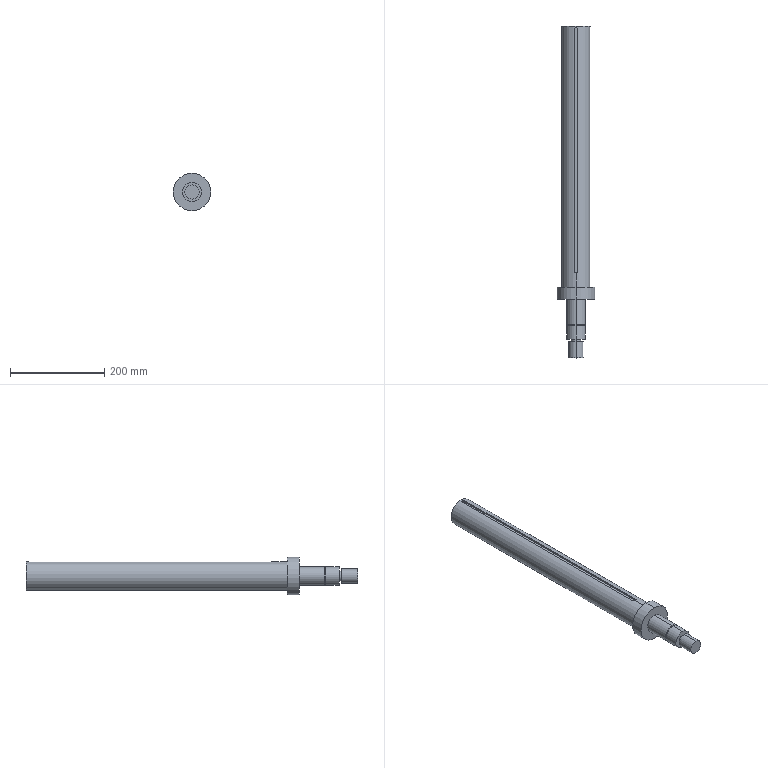Part | SolidWorks | features ICE 3, Revolution 1 | 1 solid | 30 faces | box 80 x 705.59 x 80 mm | volume 1778352 mm3 | cylinder 18 | plane 12 | commonest cylinder face diameters 30 x4 40 x4 8 x2 20 x2 36 x2 60 x2
STEP:
#1=CARTESIAN_POINT('',(0.,411.976,-15.));
#2=VERTEX_POINT('',#1);
#3=CARTESIAN_POINT('',(0.,411.976,15.));
#4=VERTEX_POINT('',#3);
#5=CARTESIAN_POINT('',(0.,411.976,0.));
#6=DIRECTION('',(0.,1.,0.));
#7=DIRECTION('',(0.,0.,1.));
#8=AXIS2_PLACEMENT_3D('',#5,#6,#7);
#9=CIRCLE('',#8,15.);
#10=EDGE_CURVE('',#2,#4,#9,.T.);
#11=ORIENTED_EDGE('',*,*,#10,.F.);
#12=CARTESIAN_POINT('',(0.,461.976,-15.));
#13=VERTEX_POINT('',#12);
#14=CARTESIAN_POINT('',(0.,411.976,-15.));
#15=DIRECTION('',(0.,1.,0.));
#16=VECTOR('',#15,1000.);
#17=LINE('',#14,#16);
#18=EDGE_CURVE('',#2,#13,#17,.T.);
#19=ORIENTED_EDGE('',*,*,#18,.T.);
#20=CARTESIAN_POINT('',(0.,461.976,15.));
#21=VERTEX_POINT('',#20);
#22=CARTESIAN_POINT('',(0.,461.976,0.));
#23=DIRECTION('',(0.,1.,0.));
#24=DIRECTION('',(0.,0.,1.));
#25=AXIS2_PLACEMENT_3D('',#22,#23,#24);
#26=CIRCLE('',#25,15.);
#27=EDGE_CURVE('',#13,#21,#26,.T.);
#28=ORIENTED_EDGE('',*,*,#27,.T.);
#29=CARTESIAN_POINT('',(0.,411.976,15.));
#30=DIRECTION('',(0.,1.,0.));
#31=VECTOR('',#30,1000.);
#32=LINE('',#29,#31);
#33=EDGE_CURVE('',#4,#21,#32,.T.);
#34=ORIENTED_EDGE('',*,*,#33,.F.);
#35=EDGE_LOOP('',(#11,#19,#28,#34));
#36=FACE_OUTER_BOUND('',#35,.T.);
#37=CARTESIAN_POINT('',(0.,411.976,0.));
#38=DIRECTION('',(0.,1.,0.));
#39=DIRECTION('',(0.,0.,1.));
#40=AXIS2_PLACEMENT_3D('',#37,#38,#39);
#41=CYLINDRICAL_SURFACE('',#40,15.);
#42=ADVANCED_FACE('',(#36),#41,.F.);
#43=CARTESIAN_POINT('',(0.,-118.614,40.));
#44=VERTEX_POINT('',#43);
#45=CARTESIAN_POINT('',(0.,-118.614,-40.));
#46=VERTEX_POINT('',#45);
#47=CARTESIAN_POINT('',(0.,-118.614,0.));
#48=DIRECTION('',(0.,1.,0.));
#49=DIRECTION('',(0.,0.,1.));
#50=AXIS2_PLACEMENT_3D('',#47,#48,#49);
#51=CIRCLE('',#50,40.);
#52=EDGE_CURVE('',#44,#46,#51,.T.);
#53=ORIENTED_EDGE('',*,*,#52,.T.);
#54=CARTESIAN_POINT('',(0.,-93.614,-40.));
#55=VERTEX_POINT('',#54);
#56=CARTESIAN_POINT('',(0.,247.86,-40.));
#57=DIRECTION('',(0.,1.,0.));
#58=VECTOR('',#57,1000.);
#59=LINE('',#56,#58);
#60=EDGE_CURVE('',#46,#55,#59,.T.);
#61=ORIENTED_EDGE('',*,*,#60,.T.);
#62=CARTESIAN_POINT('',(0.,-93.614,40.));
#63=VERTEX_POINT('',#62);
#64=CARTESIAN_POINT('',(0.,-93.614,0.));
#65=DIRECTION('',(0.,1.,0.));
#66=DIRECTION('',(0.,0.,1.));
#67=AXIS2_PLACEMENT_3D('',#64,#65,#66);
#68=CIRCLE('',#67,40.);
#69=EDGE_CURVE('',#63,#55,#68,.T.);
#70=ORIENTED_EDGE('',*,*,#69,.F.);
#71=CARTESIAN_POINT('',(0.,247.86,40.));
#72=DIRECTION('',(0.,1.,0.));
#73=VECTOR('',#72,1000.);
#74=LINE('',#71,#73);
#75=EDGE_CURVE('',#44,#63,#74,.T.);
#76=ORIENTED_EDGE('',*,*,#75,.F.);
#77=EDGE_LOOP('',(#53,#61,#70,#76));
#78=FACE_OUTER_BOUND('',#77,.T.);
#79=CARTESIAN_POINT('',(0.,247.86,0.));
#80=DIRECTION('',(0.,1.,0.));
#81=DIRECTION('',(0.,0.,1.));
#82=AXIS2_PLACEMENT_3D('',#79,#80,#81);
#83=CYLINDRICAL_SURFACE('',#82,40.);
#84=ADVANCED_FACE('',(#78),#83,.T.);
#85=CARTESIAN_POINT('',(0.,-171.914,20.));
#86=VERTEX_POINT('',#85);
#87=CARTESIAN_POINT('',(0.,-171.914,-20.));
#88=VERTEX_POINT('',#87);
#89=CARTESIAN_POINT('',(0.,-171.914,0.));
#90=DIRECTION('',(0.,1.,0.));
#91=DIRECTION('',(0.,0.,1.));
#92=AXIS2_PLACEMENT_3D('',#89,#90,#91);
#93=CIRCLE('',#92,20.);
#94=EDGE_CURVE('',#86,#88,#93,.T.);
#95=ORIENTED_EDGE('',*,*,#94,.T.);
#96=CARTESIAN_POINT('',(0.,-118.614,-20.));
#97=VERTEX_POINT('',#96);
#98=CARTESIAN_POINT('',(0.,247.86,-20.));
#99=DIRECTION('',(0.,1.,0.));
#100=VECTOR('',#99,1000.);
#101=LINE('',#98,#100);
#102=EDGE_CURVE('',#88,#97,#101,.T.);
#103=ORIENTED_EDGE('',*,*,#102,.T.);
#104=CARTESIAN_POINT('',(0.,-118.614,20.));
#105=VERTEX_POINT('',#104);
#106=CARTESIAN_POINT('',(0.,-118.614,0.));
#107=DIRECTION('',(0.,1.,0.));
#108=DIRECTION('',(0.,0.,1.));
#109=AXIS2_PLACEMENT_3D('',#106,#107,#108);
#110=CIRCLE('',#109,20.);
#111=EDGE_CURVE('',#105,#97,#110,.T.);
#112=ORIENTED_EDGE('',*,*,#111,.F.);
#113=CARTESIAN_POINT('',(0.,247.86,20.));
#114=DIRECTION('',(0.,1.,0.));
#115=VECTOR('',#114,1000.);
#116=LINE('',#113,#115);
#117=EDGE_CURVE('',#86,#105,#116,.T.);
#118=ORIENTED_EDGE('',*,*,#117,.F.);
#119=EDGE_LOOP('',(#95,#103,#112,#118));
#120=FACE_OUTER_BOUND('',#119,.T.);
#121=CARTESIAN_POINT('',(0.,247.86,0.));
#122=DIRECTION('',(0.,1.,0.));
#123=DIRECTION('',(0.,0.,1.));
#124=AXIS2_PLACEMENT_3D('',#121,#122,#123);
#125=CYLINDRICAL_SURFACE('',#124,20.);
#126=ADVANCED_FACE('',(#120),#125,.T.);
#127=CARTESIAN_POINT('',(0.,-174.914,18.));
#128=VERTEX_POINT('',#127);
#129=CARTESIAN_POINT('',(0.,-174.914,-18.));
#130=VERTEX_POINT('',#129);
#131=CARTESIAN_POINT('',(0.,-174.914,0.));
#132=DIRECTION('',(0.,1.,0.));
#133=DIRECTION('',(0.,0.,1.));
#134=AXIS2_PLACEMENT_3D('',#131,#132,#133);
#135=CIRCLE('',#134,18.);
#136=EDGE_CURVE('',#128,#130,#135,.T.);
#137=ORIENTED_EDGE('',*,*,#136,.T.);
#138=CARTESIAN_POINT('',(0.,-171.914,-18.));
#139=VERTEX_POINT('',#138);
#140=CARTESIAN_POINT('',(0.,247.86,-18.));
#141=DIRECTION('',(0.,1.,0.));
#142=VECTOR('',#141,1000.);
#143=LINE('',#140,#142);
#144=EDGE_CURVE('',#130,#139,#143,.T.);
#145=ORIENTED_EDGE('',*,*,#144,.T.);
#146=CARTESIAN_POINT('',(0.,-171.914,18.));
#147=VERTEX_POINT('',#146);
#148=CARTESIAN_POINT('',(0.,-171.914,0.));
#149=DIRECTION('',(0.,1.,0.));
#150=DIRECTION('',(0.,0.,1.));
#151=AXIS2_PLACEMENT_3D('',#148,#149,#150);
#152=CIRCLE('',#151,18.);
#153=EDGE_CURVE('',#147,#139,#152,.T.);
#154=ORIENTED_EDGE('',*,*,#153,.F.);
#155=CARTESIAN_POINT('',(0.,247.86,18.));
#156=DIRECTION('',(0.,1.,0.));
#157=VECTOR('',#156,1000.);
#158=LINE('',#155,#157);
#159=EDGE_CURVE('',#128,#147,#158,.T.);
#160=ORIENTED_EDGE('',*,*,#159,.F.);
#161=EDGE_LOOP('',(#137,#145,#154,#160));
#162=FACE_OUTER_BOUND('',#161,.T.);
#163=CARTESIAN_POINT('',(0.,247.86,0.));
#164=DIRECTION('',(0.,1.,0.));
#165=DIRECTION('',(0.,0.,1.));
#166=AXIS2_PLACEMENT_3D('',#163,#164,#165);
#167=CYLINDRICAL_SURFACE('',#166,18.);
#168=ADVANCED_FACE('',(#162),#167,.T.);
#169=CARTESIAN_POINT('',(0.,-203.614,20.));
#170=VERTEX_POINT('',#169);
#171=CARTESIAN_POINT('',(0.,-203.614,-20.));
#172=VERTEX_POINT('',#171);
#173=CARTESIAN_POINT('',(0.,-203.614,0.));
#174=DIRECTION('',(0.,1.,0.));
#175=DIRECTION('',(0.,0.,1.));
#176=AXIS2_PLACEMENT_3D('',#173,#174,#175);
#177=CIRCLE('',#176,20.);
#178=EDGE_CURVE('',#170,#172,#177,.T.);
#179=ORIENTED_EDGE('',*,*,#178,.T.);
#180=CARTESIAN_POINT('',(0.,-174.914,-20.));
#181=VERTEX_POINT('',#180);
#182=CARTESIAN_POINT('',(0.,247.86,-20.));
#183=DIRECTION('',(0.,1.,0.));
#184=VECTOR('',#183,1000.);
#185=LINE('',#182,#184);
#186=EDGE_CURVE('',#172,#181,#185,.T.);
#187=ORIENTED_EDGE('',*,*,#186,.T.);
#188=CARTESIAN_POINT('',(0.,-174.914,20.));
#189=VERTEX_POINT('',#188);
#190=CARTESIAN_POINT('',(0.,-174.914,0.));
#191=DIRECTION('',(0.,1.,0.));
#192=DIRECTION('',(0.,0.,1.));
#193=AXIS2_PLACEMENT_3D('',#190,#191,#192);
#194=CIRCLE('',#193,20.);
#195=EDGE_CURVE('',#189,#181,#194,.T.);
#196=ORIENTED_EDGE('',*,*,#195,.F.);
#197=CARTESIAN_POINT('',(0.,247.86,20.));
#198=DIRECTION('',(0.,1.,0.));
#199=VECTOR('',#198,1000.);
#200=LINE('',#197,#199);
#201=EDGE_CURVE('',#170,#189,#200,.T.);
#202=ORIENTED_EDGE('',*,*,#201,.F.);
#203=EDGE_LOOP('',(#179,#187,#196,#202));
#204=FACE_OUTER_BOUND('',#203,.T.);
#205=CARTESIAN_POINT('',(0.,247.86,0.));
#206=DIRECTION('',(0.,1.,0.));
#207=DIRECTION('',(0.,0.,1.));
#208=AXIS2_PLACEMENT_3D('',#205,#206,#207);
#209=CYLINDRICAL_SURFACE('',#208,20.);
#210=ADVANCED_FACE('',(#204),#209,.T.);
#211=CARTESIAN_POINT('',(0.,-208.614,10.));
#212=VERTEX_POINT('',#211);
#213=CARTESIAN_POINT('',(0.,-208.614,-10.));
#214=VERTEX_POINT('',#213);
#215=CARTESIAN_POINT('',(0.,-208.614,0.));
#216=DIRECTION('',(0.,1.,0.));
#217=DIRECTION('',(0.,0.,1.));
#218=AXIS2_PLACEMENT_3D('',#215,#216,#217);
#219=CIRCLE('',#218,10.);
#220=EDGE_CURVE('',#212,#214,#219,.T.);
#221=ORIENTED_EDGE('',*,*,#220,.T.);
#222=CARTESIAN_POINT('',(0.,-203.614,-10.));
#223=VERTEX_POINT('',#222);
#224=CARTESIAN_POINT('',(0.,247.86,-10.));
#225=DIRECTION('',(0.,1.,0.));
#226=VECTOR('',#225,1000.);
#227=LINE('',#224,#226);
#228=EDGE_CURVE('',#214,#223,#227,.T.);
#229=ORIENTED_EDGE('',*,*,#228,.T.);
#230=CARTESIAN_POINT('',(0.,-203.614,10.));
#231=VERTEX_POINT('',#230);
#232=CARTESIAN_POINT('',(0.,-203.614,0.));
#233=DIRECTION('',(0.,1.,0.));
#234=DIRECTION('',(0.,0.,1.));
#235=AXIS2_PLACEMENT_3D('',#232,#233,#234);
#236=CIRCLE('',#235,10.);
#237=EDGE_CURVE('',#231,#223,#236,.T.);
#238=ORIENTED_EDGE('',*,*,#237,.F.);
#239=CARTESIAN_POINT('',(0.,247.86,10.));
#240=DIRECTION('',(0.,1.,0.));
#241=VECTOR('',#240,1000.);
#242=LINE('',#239,#241);
#243=EDGE_CURVE('',#212,#231,#242,.T.);
#244=ORIENTED_EDGE('',*,*,#243,.F.);
#245=EDGE_LOOP('',(#221,#229,#238,#244));
#246=FACE_OUTER_BOUND('',#245,.T.);
#247=CARTESIAN_POINT('',(0.,247.86,0.));
#248=DIRECTION('',(0.,1.,0.));
#249=DIRECTION('',(0.,0.,1.));
#250=AXIS2_PLACEMENT_3D('',#247,#248,#249);
#251=CYLINDRICAL_SURFACE('',#250,10.);
#252=ADVANCED_FACE('',(#246),#251,.T.);
#253=CARTESIAN_POINT('',(0.,-243.614,15.));
#254=VERTEX_POINT('',#253);
#255=CARTESIAN_POINT('',(0.,-243.614,-15.));
#256=VERTEX_POINT('',#255);
#257=CARTESIAN_POINT('',(0.,-243.614,0.));
#258=DIRECTION('',(0.,1.,0.));
#259=DIRECTION('',(0.,0.,1.));
#260=AXIS2_PLACEMENT_3D('',#257,#258,#259);
#261=CIRCLE('',#260,15.);
#262=EDGE_CURVE('',#254,#256,#261,.T.);
#263=ORIENTED_EDGE('',*,*,#262,.T.);
#264=CARTESIAN_POINT('',(0.,-208.614,-15.));
#265=VERTEX_POINT('',#264);
#266=CARTESIAN_POINT('',(0.,247.86,-15.));
#267=DIRECTION('',(0.,1.,0.));
#268=VECTOR('',#267,1000.);
#269=LINE('',#266,#268);
#270=EDGE_CURVE('',#256,#265,#269,.T.);
#271=ORIENTED_EDGE('',*,*,#270,.T.);
#272=CARTESIAN_POINT('',(0.,-208.614,15.));
#273=VERTEX_POINT('',#272);
#274=CARTESIAN_POINT('',(0.,-208.614,0.));
#275=DIRECTION('',(0.,1.,0.));
#276=DIRECTION('',(0.,0.,1.));
#277=AXIS2_PLACEMENT_3D('',#274,#275,#276);
#278=CIRCLE('',#277,15.);
#279=EDGE_CURVE('',#273,#265,#278,.T.);
#280=ORIENTED_EDGE('',*,*,#279,.F.);
#281=CARTESIAN_POINT('',(0.,247.86,15.));
#282=DIRECTION('',(0.,1.,0.));
#283=VECTOR('',#282,1000.);
#284=LINE('',#281,#283);
#285=EDGE_CURVE('',#254,#273,#284,.T.);
#286=ORIENTED_EDGE('',*,*,#285,.F.);
#287=EDGE_LOOP('',(#263,#271,#280,#286));
#288=FACE_OUTER_BOUND('',#287,.T.);
#289=CARTESIAN_POINT('',(0.,247.86,0.));
#290=DIRECTION('',(0.,1.,0.));
#291=DIRECTION('',(0.,0.,1.));
#292=AXIS2_PLACEMENT_3D('',#289,#290,#291);
#293=CYLINDRICAL_SURFACE('',#292,15.);
#294=ADVANCED_FACE('',(#288),#293,.T.);
#295=CARTESIAN_POINT('',(0.,-93.614,30.));
#296=VERTEX_POINT('',#295);
#297=CARTESIAN_POINT('',(0.,-93.614,-30.));
#298=VERTEX_POINT('',#297);
#299=CARTESIAN_POINT('',(0.,-93.614,0.));
#300=DIRECTION('',(0.,1.,0.));
#301=DIRECTION('',(0.,0.,1.));
#302=AXIS2_PLACEMENT_3D('',#299,#300,#301);
#303=CIRCLE('',#302,30.);
#304=EDGE_CURVE('',#296,#298,#303,.T.);
#305=ORIENTED_EDGE('',*,*,#304,.T.);
#306=CARTESIAN_POINT('',(0.,461.976,-30.));
#307=VERTEX_POINT('',#306);
#308=CARTESIAN_POINT('',(0.,247.86,-30.));
#309=DIRECTION('',(0.,1.,0.));
#310=VECTOR('',#309,1000.);
#311=LINE('',#308,#310);
#312=EDGE_CURVE('',#298,#307,#311,.T.);
#313=ORIENTED_EDGE('',*,*,#312,.T.);
#314=CARTESIAN_POINT('',(0.,461.976,30.));
#315=VERTEX_POINT('',#314);
#316=CARTESIAN_POINT('',(0.,461.976,0.));
#317=DIRECTION('',(0.,1.,0.));
#318=DIRECTION('',(0.,0.,1.));
#319=AXIS2_PLACEMENT_3D('',#316,#317,#318);
#320=CIRCLE('',#319,30.);
#321=EDGE_CURVE('',#315,#307,#320,.T.);
#322=ORIENTED_EDGE('',*,*,#321,.F.);
#323=CARTESIAN_POINT('',(0.,458.476,30.));
#324=VERTEX_POINT('',#323);
#325=CARTESIAN_POINT('',(0.,247.86,30.));
#326=DIRECTION('',(0.,1.,0.));
#327=VECTOR('',#326,1000.);
#328=LINE('',#325,#327);
#329=EDGE_CURVE('',#324,#315,#328,.T.);
#330=ORIENTED_EDGE('',*,*,#329,.F.);
#331=CARTESIAN_POINT('',(4.,454.476,29.732));
#332=VERTEX_POINT('',#331);
#333=CARTESIAN_POINT('',(4.,454.476,29.732));
#334=CARTESIAN_POINT('',(4.,454.74,29.732));
#335=CARTESIAN_POINT('',(3.974,455.001,29.736));
#336=CARTESIAN_POINT('',(3.872,455.512,29.749));
#337=CARTESIAN_POINT('',(3.795,455.767,29.759));
#338=CARTESIAN_POINT('',(3.594,456.251,29.784));
#339=CARTESIAN_POINT('',(3.471,456.481,29.799));
#340=CARTESIAN_POINT('',(3.181,456.915,29.831));
#341=CARTESIAN_POINT('',(3.012,457.121,29.849));
#342=CARTESIAN_POINT('',(2.643,457.49,29.884));
#343=CARTESIAN_POINT('',(2.442,457.655,29.901));
#344=CARTESIAN_POINT('',(2.004,457.947,29.934));
#345=CARTESIAN_POINT('',(1.772,458.071,29.949));
#346=CARTESIAN_POINT('',(1.29,458.271,29.973));
#347=CARTESIAN_POINT('',(1.038,458.348,29.983));
#348=CARTESIAN_POINT('',(0.5211,458.45,29.997));
#349=CARTESIAN_POINT('',(0.2613,458.476,30.));
#350=CARTESIAN_POINT('',(0.,458.476,30.));
#351=B_SPLINE_CURVE_WITH_KNOTS('',3,(#333,#334,#335,#336,#337,#338,#339,#340,#341,#342,#343,#344,#345,#346,#347,#348,#349,#350),.UNSPECIFIED.,.F.,.F.,(4,2,2,2,2,2,2,2,4),(0.,0.0007827,0.001565,0.002348,0.003131,0.003913,0.004696,0.005479,0.006261),.UNSPECIFIED.);
#352=EDGE_CURVE('',#332,#324,#351,.T.);
#353=ORIENTED_EDGE('',*,*,#352,.F.);
#354=CARTESIAN_POINT('',(4.,-58.114,29.732));
#355=VERTEX_POINT('',#354);
#356=CARTESIAN_POINT('',(4.,247.86,29.732));
#357=DIRECTION('',(0.,-1.,0.));
#358=VECTOR('',#357,1000.);
#359=LINE('',#356,#358);
#360=EDGE_CURVE('',#332,#355,#359,.T.);
#361=ORIENTED_EDGE('',*,*,#360,.T.);
#362=CARTESIAN_POINT('',(0.,-62.114,30.));
#363=VERTEX_POINT('',#362);
#364=CARTESIAN_POINT('',(0.,-62.114,30.));
#365=CARTESIAN_POINT('',(0.261,-62.114,30.));
#366=CARTESIAN_POINT('',(0.5262,-62.088,29.996));
#367=CARTESIAN_POINT('',(1.039,-61.986,29.983));
#368=CARTESIAN_POINT('',(1.288,-61.91,29.973));
#369=CARTESIAN_POINT('',(1.773,-61.71,29.949));
#370=CARTESIAN_POINT('',(2.006,-61.584,29.934));
#371=CARTESIAN_POINT('',(2.439,-61.295,29.901));
#372=CARTESIAN_POINT('',(2.641,-61.13,29.884));
#373=CARTESIAN_POINT('',(3.014,-60.757,29.849));
#374=CARTESIAN_POINT('',(3.179,-60.555,29.831));
#375=CARTESIAN_POINT('',(3.469,-60.123,29.799));
#376=CARTESIAN_POINT('',(3.594,-59.889,29.784));
#377=CARTESIAN_POINT('',(3.795,-59.405,29.759));
#378=CARTESIAN_POINT('',(3.871,-59.156,29.749));
#379=CARTESIAN_POINT('',(3.973,-58.643,29.736));
#380=CARTESIAN_POINT('',(4.,-58.379,29.732));
#381=CARTESIAN_POINT('',(4.,-58.114,29.732));
#382=B_SPLINE_CURVE_WITH_KNOTS('',3,(#364,#365,#366,#367,#368,#369,#370,#371,#372,#373,#374,#375,#376,#377,#378,#379,#380,#381),.UNSPECIFIED.,.F.,.F.,(4,2,2,2,2,2,2,2,4),(0.006261,0.007043,0.007825,0.008607,0.009389,0.01017,0.01095,0.01173,0.01252),.UNSPECIFIED.);
#383=EDGE_CURVE('',#363,#355,#382,.T.);
#384=ORIENTED_EDGE('',*,*,#383,.F.);
#385=CARTESIAN_POINT('',(0.,247.86,30.));
#386=DIRECTION('',(0.,1.,0.));
#387=VECTOR('',#386,1000.);
#388=LINE('',#385,#387);
#389=EDGE_CURVE('',#296,#363,#388,.T.);
#390=ORIENTED_EDGE('',*,*,#389,.F.);
#391=EDGE_LOOP('',(#305,#313,#322,#330,#353,#361,#384,#390));
#392=FACE_OUTER_BOUND('',#391,.T.);
#393=CARTESIAN_POINT('',(0.,247.86,0.));
#394=DIRECTION('',(0.,1.,0.));
#395=DIRECTION('',(0.,0.,1.));
#396=AXIS2_PLACEMENT_3D('',#393,#394,#395);
#397=CYLINDRICAL_SURFACE('',#396,30.);
#398=ADVANCED_FACE('',(#392),#397,.T.);
#399=ORIENTED_EDGE('',*,*,#312,.F.);
#400=CARTESIAN_POINT('',(0.,-93.614,0.));
#401=DIRECTION('',(0.,1.,0.));
#402=DIRECTION('',(0.,0.,1.));
#403=AXIS2_PLACEMENT_3D('',#400,#401,#402);
#404=CIRCLE('',#403,30.);
#405=EDGE_CURVE('',#298,#296,#404,.T.);
#406=ORIENTED_EDGE('',*,*,#405,.T.);
#407=ORIENTED_EDGE('',*,*,#389,.T.);
#408=CARTESIAN_POINT('',(-4.,-58.114,29.732));
#409=VERTEX_POINT('',#408);
#410=CARTESIAN_POINT('',(-4.,-58.114,29.732));
#411=CARTESIAN_POINT('',(-4.,-58.379,29.732));
#412=CARTESIAN_POINT('',(-3.974,-58.639,29.736));
#413=CARTESIAN_POINT('',(-3.872,-59.151,29.749));
#414=CARTESIAN_POINT('',(-3.795,-59.405,29.759));
#415=CARTESIAN_POINT('',(-3.594,-59.89,29.784));
#416=CARTESIAN_POINT('',(-3.471,-60.119,29.799));
#417=CARTESIAN_POINT('',(-3.181,-60.554,29.831));
#418=CARTESIAN_POINT('',(-3.012,-60.759,29.849));
#419=CARTESIAN_POINT('',(-2.643,-61.128,29.884));
#420=CARTESIAN_POINT('',(-2.442,-61.293,29.901));
#421=CARTESIAN_POINT('',(-2.004,-61.586,29.934));
#422=CARTESIAN_POINT('',(-1.772,-61.71,29.949));
#423=CARTESIAN_POINT('',(-1.29,-61.909,29.973));
#424=CARTESIAN_POINT('',(-1.038,-61.986,29.983));
#425=CARTESIAN_POINT('',(-0.5211,-62.089,29.997));
#426=CARTESIAN_POINT('',(-0.2613,-62.114,30.));
#427=CARTESIAN_POINT('',(0.,-62.114,30.));
#428=B_SPLINE_CURVE_WITH_KNOTS('',3,(#410,#411,#412,#413,#414,#415,#416,#417,#418,#419,#420,#421,#422,#423,#424,#425,#426,#427),.UNSPECIFIED.,.F.,.F.,(4,2,2,2,2,2,2,2,4),(0.,0.0007827,0.001565,0.002348,0.003131,0.003913,0.004696,0.005479,0.006261),.UNSPECIFIED.);
#429=EDGE_CURVE('',#409,#363,#428,.T.);
#430=ORIENTED_EDGE('',*,*,#429,.F.);
#431=CARTESIAN_POINT('',(-4.,454.476,29.732));
#432=VERTEX_POINT('',#431);
#433=CARTESIAN_POINT('',(-4.,247.86,29.732));
#434=DIRECTION('',(0.,1.,0.));
#435=VECTOR('',#434,1000.);
#436=LINE('',#433,#435);
#437=EDGE_CURVE('',#409,#432,#436,.T.);
#438=ORIENTED_EDGE('',*,*,#437,.T.);
#439=CARTESIAN_POINT('',(0.,458.476,30.));
#440=CARTESIAN_POINT('',(-0.261,458.476,30.));
#441=CARTESIAN_POINT('',(-0.5262,458.45,29.996));
#442=CARTESIAN_POINT('',(-1.039,458.347,29.983));
#443=CARTESIAN_POINT('',(-1.288,458.272,29.973));
#444=CARTESIAN_POINT('',(-1.773,458.071,29.949));
#445=CARTESIAN_POINT('',(-2.006,457.946,29.934));
#446=CARTESIAN_POINT('',(-2.439,457.657,29.901));
#447=CARTESIAN_POINT('',(-2.641,457.491,29.884));
#448=CARTESIAN_POINT('',(-3.014,457.119,29.849));
#449=CARTESIAN_POINT('',(-3.179,456.917,29.831));
#450=CARTESIAN_POINT('',(-3.469,456.484,29.799));
#451=CARTESIAN_POINT('',(-3.594,456.251,29.784));
#452=CARTESIAN_POINT('',(-3.795,455.767,29.759));
#453=CARTESIAN_POINT('',(-3.871,455.518,29.749));
#454=CARTESIAN_POINT('',(-3.973,455.005,29.736));
#455=CARTESIAN_POINT('',(-4.,454.74,29.732));
#456=CARTESIAN_POINT('',(-4.,454.476,29.732));
#457=B_SPLINE_CURVE_WITH_KNOTS('',3,(#439,#440,#441,#442,#443,#444,#445,#446,#447,#448,#449,#450,#451,#452,#453,#454,#455,#456),.UNSPECIFIED.,.F.,.F.,(4,2,2,2,2,2,2,2,4),(0.006261,0.007043,0.007825,0.008607,0.009389,0.01017,0.01095,0.01173,0.01252),.UNSPECIFIED.);
#458=EDGE_CURVE('',#324,#432,#457,.T.);
#459=ORIENTED_EDGE('',*,*,#458,.F.);
#460=ORIENTED_EDGE('',*,*,#329,.T.);
#461=CARTESIAN_POINT('',(0.,461.976,0.));
#462=DIRECTION('',(0.,1.,0.));
#463=DIRECTION('',(0.,0.,1.));
#464=AXIS2_PLACEMENT_3D('',#461,#462,#463);
#465=CIRCLE('',#464,30.);
#466=EDGE_CURVE('',#307,#315,#465,.T.);
#467=ORIENTED_EDGE('',*,*,#466,.F.);
#468=EDGE_LOOP('',(#399,#406,#407,#430,#438,#459,#460,#467));
#469=FACE_OUTER_BOUND('',#468,.T.);
#470=CARTESIAN_POINT('',(0.,247.86,0.));
#471=DIRECTION('',(0.,1.,0.));
#472=DIRECTION('',(0.,0.,1.));
#473=AXIS2_PLACEMENT_3D('',#470,#471,#472);
#474=CYLINDRICAL_SURFACE('',#473,30.);
#475=ADVANCED_FACE('',(#469),#474,.T.);
#476=ORIENTED_EDGE('',*,*,#262,.F.);
#477=CARTESIAN_POINT('',(0.,-243.614,0.));
#478=DIRECTION('',(0.,1.,0.));
#479=DIRECTION('',(0.,0.,1.));
#480=AXIS2_PLACEMENT_3D('',#477,#478,#479);
#481=CIRCLE('',#480,15.);
#482=EDGE_CURVE('',#256,#254,#481,.T.);
#483=ORIENTED_EDGE('',*,*,#482,.F.);
#484=EDGE_LOOP('',(#476,#483));
#485=FACE_OUTER_BOUND('',#484,.T.);
#486=CARTESIAN_POINT('',(0.,-243.614,0.));
#487=DIRECTION('',(0.,1.,0.));
#488=DIRECTION('',(0.,0.,1.));
#489=AXIS2_PLACEMENT_3D('',#486,#487,#488);
#490=PLANE('',#489);
#491=ADVANCED_FACE('',(#485),#490,.F.);
#492=ORIENTED_EDGE('',*,*,#270,.F.);
#493=ORIENTED_EDGE('',*,*,#482,.T.);
#494=ORIENTED_EDGE('',*,*,#285,.T.);
#495=CARTESIAN_POINT('',(0.,-208.614,0.));
#496=DIRECTION('',(0.,1.,0.));
#497=DIRECTION('',(0.,0.,1.));
#498=AXIS2_PLACEMENT_3D('',#495,#496,#497);
#499=CIRCLE('',#498,15.);
#500=EDGE_CURVE('',#265,#273,#499,.T.);
#501=ORIENTED_EDGE('',*,*,#500,.F.);
#502=EDGE_LOOP('',(#492,#493,#494,#501));
#503=FACE_OUTER_BOUND('',#502,.T.);
#504=CARTESIAN_POINT('',(0.,247.86,0.));
#505=DIRECTION('',(0.,1.,0.));
#506=DIRECTION('',(0.,0.,1.));
#507=AXIS2_PLACEMENT_3D('',#504,#505,#506);
#508=CYLINDRICAL_SURFACE('',#507,15.);
#509=ADVANCED_FACE('',(#503),#508,.T.);
#510=ORIENTED_EDGE('',*,*,#220,.F.);
#511=CARTESIAN_POINT('',(0.,-208.614,0.));
#512=DIRECTION('',(0.,1.,0.));
#513=DIRECTION('',(0.,0.,1.));
#514=AXIS2_PLACEMENT_3D('',#511,#512,#513);
#515=CIRCLE('',#514,10.);
#516=EDGE_CURVE('',#214,#212,#515,.T.);
#517=ORIENTED_EDGE('',*,*,#516,.F.);
#518=EDGE_LOOP('',(#510,#517));
#519=FACE_BOUND('',#518,.T.);
#520=ORIENTED_EDGE('',*,*,#279,.T.);
#521=ORIENTED_EDGE('',*,*,#500,.T.);
#522=EDGE_LOOP('',(#520,#521));
#523=FACE_OUTER_BOUND('',#522,.T.);
#524=CARTESIAN_POINT('',(15.,-208.614,0.));
#525=DIRECTION('',(0.,-1.,0.));
#526=DIRECTION('',(0.,0.,-1.));
#527=AXIS2_PLACEMENT_3D('',#524,#525,#526);
#528=PLANE('',#527);
#529=ADVANCED_FACE('',(#519,#523),#528,.F.);
#530=ORIENTED_EDGE('',*,*,#228,.F.);
#531=ORIENTED_EDGE('',*,*,#516,.T.);
#532=ORIENTED_EDGE('',*,*,#243,.T.);
#533=CARTESIAN_POINT('',(0.,-203.614,0.));
#534=DIRECTION('',(0.,1.,0.));
#535=DIRECTION('',(0.,0.,1.));
#536=AXIS2_PLACEMENT_3D('',#533,#534,#535);
#537=CIRCLE('',#536,10.);
#538=EDGE_CURVE('',#223,#231,#537,.T.);
#539=ORIENTED_EDGE('',*,*,#538,.F.);
#540=EDGE_LOOP('',(#530,#531,#532,#539));
#541=FACE_OUTER_BOUND('',#540,.T.);
#542=CARTESIAN_POINT('',(0.,247.86,0.));
#543=DIRECTION('',(0.,1.,0.));
#544=DIRECTION('',(0.,0.,1.));
#545=AXIS2_PLACEMENT_3D('',#542,#543,#544);
#546=CYLINDRICAL_SURFACE('',#545,10.);
#547=ADVANCED_FACE('',(#541),#546,.T.);
#548=ORIENTED_EDGE('',*,*,#178,.F.);
#549=CARTESIAN_POINT('',(0.,-203.614,0.));
#550=DIRECTION('',(0.,1.,0.));
#551=DIRECTION('',(0.,0.,1.));
#552=AXIS2_PLACEMENT_3D('',#549,#550,#551);
#553=CIRCLE('',#552,20.);
#554=EDGE_CURVE('',#172,#170,#553,.T.);
#555=ORIENTED_EDGE('',*,*,#554,.F.);
#556=EDGE_LOOP('',(#548,#555));
#557=FACE_OUTER_BOUND('',#556,.T.);
#558=ORIENTED_EDGE('',*,*,#237,.T.);
#559=ORIENTED_EDGE('',*,*,#538,.T.);
#560=EDGE_LOOP('',(#558,#559));
#561=FACE_BOUND('',#560,.T.);
#562=CARTESIAN_POINT('',(10.,-203.614,0.));
#563=DIRECTION('',(0.,1.,0.));
#564=DIRECTION('',(0.,0.,1.));
#565=AXIS2_PLACEMENT_3D('',#562,#563,#564);
#566=PLANE('',#565);
#567=ADVANCED_FACE('',(#557,#561),#566,.F.);
#568=ORIENTED_EDGE('',*,*,#186,.F.);
#569=ORIENTED_EDGE('',*,*,#554,.T.);
#570=ORIENTED_EDGE('',*,*,#201,.T.);
#571=CARTESIAN_POINT('',(0.,-174.914,0.));
#572=DIRECTION('',(0.,1.,0.));
#573=DIRECTION('',(0.,0.,1.));
#574=AXIS2_PLACEMENT_3D('',#571,#572,#573);
#575=CIRCLE('',#574,20.);
#576=EDGE_CURVE('',#181,#189,#575,.T.);
#577=ORIENTED_EDGE('',*,*,#576,.F.);
#578=EDGE_LOOP('',(#568,#569,#570,#577));
#579=FACE_OUTER_BOUND('',#578,.T.);
#580=CARTESIAN_POINT('',(0.,247.86,0.));
#581=DIRECTION('',(0.,1.,0.));
#582=DIRECTION('',(0.,0.,1.));
#583=AXIS2_PLACEMENT_3D('',#580,#581,#582);
#584=CYLINDRICAL_SURFACE('',#583,20.);
#585=ADVANCED_FACE('',(#579),#584,.T.);
#586=ORIENTED_EDGE('',*,*,#136,.F.);
#587=CARTESIAN_POINT('',(0.,-174.914,0.));
#588=DIRECTION('',(0.,1.,0.));
#589=DIRECTION('',(0.,0.,1.));
#590=AXIS2_PLACEMENT_3D('',#587,#588,#589);
#591=CIRCLE('',#590,18.);
#592=EDGE_CURVE('',#130,#128,#591,.T.);
#593=ORIENTED_EDGE('',*,*,#592,.F.);
#594=EDGE_LOOP('',(#586,#593));
#595=FACE_BOUND('',#594,.T.);
#596=ORIENTED_EDGE('',*,*,#195,.T.);
#597=ORIENTED_EDGE('',*,*,#576,.T.);
#598=EDGE_LOOP('',(#596,#597));
#599=FACE_OUTER_BOUND('',#598,.T.);
#600=CARTESIAN_POINT('',(20.,-174.914,0.));
#601=DIRECTION('',(0.,-1.,0.));
#602=DIRECTION('',(0.,0.,-1.));
#603=AXIS2_PLACEMENT_3D('',#600,#601,#602);
#604=PLANE('',#603);
#605=ADVANCED_FACE('',(#595,#599),#604,.F.);
#606=ORIENTED_EDGE('',*,*,#144,.F.);
#607=ORIENTED_EDGE('',*,*,#592,.T.);
#608=ORIENTED_EDGE('',*,*,#159,.T.);
#609=CARTESIAN_POINT('',(0.,-171.914,0.));
#610=DIRECTION('',(0.,1.,0.));
#611=DIRECTION('',(0.,0.,1.));
#612=AXIS2_PLACEMENT_3D('',#609,#610,#611);
#613=CIRCLE('',#612,18.);
#614=EDGE_CURVE('',#139,#147,#613,.T.);
#615=ORIENTED_EDGE('',*,*,#614,.F.);
#616=EDGE_LOOP('',(#606,#607,#608,#615));
#617=FACE_OUTER_BOUND('',#616,.T.);
#618=CARTESIAN_POINT('',(0.,247.86,0.));
#619=DIRECTION('',(0.,1.,0.));
#620=DIRECTION('',(0.,0.,1.));
#621=AXIS2_PLACEMENT_3D('',#618,#619,#620);
#622=CYLINDRICAL_SURFACE('',#621,18.);
#623=ADVANCED_FACE('',(#617),#622,.T.);
#624=ORIENTED_EDGE('',*,*,#94,.F.);
#625=CARTESIAN_POINT('',(0.,-171.914,0.));
#626=DIRECTION('',(0.,1.,0.));
#627=DIRECTION('',(0.,0.,1.));
#628=AXIS2_PLACEMENT_3D('',#625,#626,#627);
#629=CIRCLE('',#628,20.);
#630=EDGE_CURVE('',#88,#86,#629,.T.);
#631=ORIENTED_EDGE('',*,*,#630,.F.);
#632=EDGE_LOOP('',(#624,#631));
#633=FACE_OUTER_BOUND('',#632,.T.);
#634=ORIENTED_EDGE('',*,*,#153,.T.);
#635=ORIENTED_EDGE('',*,*,#614,.T.);
#636=EDGE_LOOP('',(#634,#635));
#637=FACE_BOUND('',#636,.T.);
#638=CARTESIAN_POINT('',(18.,-171.914,0.));
#639=DIRECTION('',(0.,1.,0.));
#640=DIRECTION('',(0.,0.,1.));
#641=AXIS2_PLACEMENT_3D('',#638,#639,#640);
#642=PLANE('',#641);
#643=ADVANCED_FACE('',(#633,#637),#642,.F.);
#644=ORIENTED_EDGE('',*,*,#102,.F.);
#645=ORIENTED_EDGE('',*,*,#630,.T.);
#646=ORIENTED_EDGE('',*,*,#117,.T.);
#647=CARTESIAN_POINT('',(0.,-118.614,0.));
#648=DIRECTION('',(0.,1.,0.));
#649=DIRECTION('',(0.,0.,1.));
#650=AXIS2_PLACEMENT_3D('',#647,#648,#649);
#651=CIRCLE('',#650,20.);
#652=EDGE_CURVE('',#97,#105,#651,.T.);
#653=ORIENTED_EDGE('',*,*,#652,.F.);
#654=EDGE_LOOP('',(#644,#645,#646,#653));
#655=FACE_OUTER_BOUND('',#654,.T.);
#656=CARTESIAN_POINT('',(0.,247.86,0.));
#657=DIRECTION('',(0.,1.,0.));
#658=DIRECTION('',(0.,0.,1.));
#659=AXIS2_PLACEMENT_3D('',#656,#657,#658);
#660=CYLINDRICAL_SURFACE('',#659,20.);
#661=ADVANCED_FACE('',(#655),#660,.T.);
#662=ORIENTED_EDGE('',*,*,#52,.F.);
#663=CARTESIAN_POINT('',(0.,-118.614,0.));
#664=DIRECTION('',(0.,1.,0.));
#665=DIRECTION('',(0.,0.,1.));
#666=AXIS2_PLACEMENT_3D('',#663,#664,#665);
#667=CIRCLE('',#666,40.);
#668=EDGE_CURVE('',#46,#44,#667,.T.);
#669=ORIENTED_EDGE('',*,*,#668,.F.);
#670=EDGE_LOOP('',(#662,#669));
#671=FACE_OUTER_BOUND('',#670,.T.);
#672=ORIENTED_EDGE('',*,*,#111,.T.);
#673=ORIENTED_EDGE('',*,*,#652,.T.);
#674=EDGE_LOOP('',(#672,#673));
#675=FACE_BOUND('',#674,.T.);
#676=CARTESIAN_POINT('',(20.,-118.614,0.));
#677=DIRECTION('',(0.,1.,0.));
#678=DIRECTION('',(0.,0.,1.));
#679=AXIS2_PLACEMENT_3D('',#676,#677,#678);
#680=PLANE('',#679);
#681=ADVANCED_FACE('',(#671,#675),#680,.F.);
#682=ORIENTED_EDGE('',*,*,#60,.F.);
#683=ORIENTED_EDGE('',*,*,#668,.T.);
#684=ORIENTED_EDGE('',*,*,#75,.T.);
#685=CARTESIAN_POINT('',(0.,-93.614,0.));
#686=DIRECTION('',(0.,1.,0.));
#687=DIRECTION('',(0.,0.,1.));
#688=AXIS2_PLACEMENT_3D('',#685,#686,#687);
#689=CIRCLE('',#688,40.);
#690=EDGE_CURVE('',#55,#63,#689,.T.);
#691=ORIENTED_EDGE('',*,*,#690,.F.);
#692=EDGE_LOOP('',(#682,#683,#684,#691));
#693=FACE_OUTER_BOUND('',#692,.T.);
#694=CARTESIAN_POINT('',(0.,247.86,0.));
#695=DIRECTION('',(0.,1.,0.));
#696=DIRECTION('',(0.,0.,1.));
#697=AXIS2_PLACEMENT_3D('',#694,#695,#696);
#698=CYLINDRICAL_SURFACE('',#697,40.);
#699=ADVANCED_FACE('',(#693),#698,.T.);
#700=ORIENTED_EDGE('',*,*,#304,.F.);
#701=ORIENTED_EDGE('',*,*,#405,.F.);
#702=EDGE_LOOP('',(#700,#701));
#703=FACE_BOUND('',#702,.T.);
#704=ORIENTED_EDGE('',*,*,#69,.T.);
#705=ORIENTED_EDGE('',*,*,#690,.T.);
#706=EDGE_LOOP('',(#704,#705));
#707=FACE_OUTER_BOUND('',#706,.T.);
#708=CARTESIAN_POINT('',(40.,-93.614,0.));
#709=DIRECTION('',(0.,-1.,0.));
#710=DIRECTION('',(0.,0.,-1.));
#711=AXIS2_PLACEMENT_3D('',#708,#709,#710);
#712=PLANE('',#711);
#713=ADVANCED_FACE('',(#703,#707),#712,.F.);
#714=CARTESIAN_POINT('',(0.,461.976,0.));
#715=DIRECTION('',(0.,1.,0.));
#716=DIRECTION('',(0.,0.,1.));
#717=AXIS2_PLACEMENT_3D('',#714,#715,#716);
#718=CIRCLE('',#717,15.);
#719=EDGE_CURVE('',#21,#13,#718,.T.);
#720=ORIENTED_EDGE('',*,*,#719,.F.);
#721=ORIENTED_EDGE('',*,*,#27,.F.);
#722=EDGE_LOOP('',(#720,#721));
#723=FACE_BOUND('',#722,.T.);
#724=ORIENTED_EDGE('',*,*,#321,.T.);
#725=ORIENTED_EDGE('',*,*,#466,.T.);
#726=EDGE_LOOP('',(#724,#725));
#727=FACE_OUTER_BOUND('',#726,.T.);
#728=CARTESIAN_POINT('',(30.,461.976,0.));
#729=DIRECTION('',(0.,-1.,0.));
#730=DIRECTION('',(0.,0.,-1.));
#731=AXIS2_PLACEMENT_3D('',#728,#729,#730);
#732=PLANE('',#731);
#733=ADVANCED_FACE('',(#723,#727),#732,.F.);
#734=ORIENTED_EDGE('',*,*,#18,.F.);
#735=CARTESIAN_POINT('',(0.,411.976,0.));
#736=DIRECTION('',(0.,1.,0.));
#737=DIRECTION('',(0.,0.,1.));
#738=AXIS2_PLACEMENT_3D('',#735,#736,#737);
#739=CIRCLE('',#738,15.);
#740=EDGE_CURVE('',#4,#2,#739,.T.);
#741=ORIENTED_EDGE('',*,*,#740,.F.);
#742=ORIENTED_EDGE('',*,*,#33,.T.);
#743=ORIENTED_EDGE('',*,*,#719,.T.);
#744=EDGE_LOOP('',(#734,#741,#742,#743));
#745=FACE_OUTER_BOUND('',#744,.T.);
#746=CARTESIAN_POINT('',(0.,411.976,0.));
#747=DIRECTION('',(0.,1.,0.));
#748=DIRECTION('',(0.,0.,1.));
#749=AXIS2_PLACEMENT_3D('',#746,#747,#748);
#750=CYLINDRICAL_SURFACE('',#749,15.);
#751=ADVANCED_FACE('',(#745),#750,.F.);
#752=ORIENTED_EDGE('',*,*,#740,.T.);
#753=ORIENTED_EDGE('',*,*,#10,.T.);
#754=EDGE_LOOP('',(#752,#753));
#755=FACE_OUTER_BOUND('',#754,.T.);
#756=CARTESIAN_POINT('',(0.,411.976,0.));
#757=DIRECTION('',(0.,1.,0.));
#758=DIRECTION('',(0.,0.,1.));
#759=AXIS2_PLACEMENT_3D('',#756,#757,#758);
#760=PLANE('',#759);
#761=ADVANCED_FACE('',(#755),#760,.T.);
#762=CARTESIAN_POINT('',(4.,454.476,26.232));
#763=VERTEX_POINT('',#762);
#764=CARTESIAN_POINT('',(4.,454.476,26.232));
#765=DIRECTION('',(0.,0.,-1.));
#766=VECTOR('',#765,1000.);
#767=LINE('',#764,#766);
#768=EDGE_CURVE('',#332,#763,#767,.T.);
#769=ORIENTED_EDGE('',*,*,#768,.T.);
#770=CARTESIAN_POINT('',(4.,-58.114,26.232));
#771=VERTEX_POINT('',#770);
#772=CARTESIAN_POINT('',(4.,-58.114,26.232));
#773=DIRECTION('',(0.,1.,0.));
#774=VECTOR('',#773,1000.);
#775=LINE('',#772,#774);
#776=EDGE_CURVE('',#771,#763,#775,.T.);
#777=ORIENTED_EDGE('',*,*,#776,.F.);
#778=CARTESIAN_POINT('',(4.,-58.114,26.232));
#779=DIRECTION('',(0.,0.,-1.));
#780=VECTOR('',#779,1000.);
#781=LINE('',#778,#780);
#782=EDGE_CURVE('',#355,#771,#781,.T.);
#783=ORIENTED_EDGE('',*,*,#782,.F.);
#784=ORIENTED_EDGE('',*,*,#360,.F.);
#785=EDGE_LOOP('',(#769,#777,#783,#784));
#786=FACE_OUTER_BOUND('',#785,.T.);
#787=CARTESIAN_POINT('',(4.,-58.114,26.232));
#788=DIRECTION('',(1.,0.,0.));
#789=DIRECTION('',(0.,0.,-1.));
#790=AXIS2_PLACEMENT_3D('',#787,#788,#789);
#791=PLANE('',#790);
#792=ADVANCED_FACE('',(#786),#791,.F.);
#793=CARTESIAN_POINT('',(-4.,-58.114,26.232));
#794=VERTEX_POINT('',#793);
#795=CARTESIAN_POINT('',(-4.,-58.114,26.232));
#796=DIRECTION('',(0.,0.,1.));
#797=VECTOR('',#796,1000.);
#798=LINE('',#795,#797);
#799=EDGE_CURVE('',#794,#409,#798,.T.);
#800=ORIENTED_EDGE('',*,*,#799,.F.);
#801=CARTESIAN_POINT('',(-4.,454.476,26.232));
#802=VERTEX_POINT('',#801);
#803=CARTESIAN_POINT('',(-4.,-58.114,26.232));
#804=DIRECTION('',(0.,1.,0.));
#805=VECTOR('',#804,1000.);
#806=LINE('',#803,#805);
#807=EDGE_CURVE('',#794,#802,#806,.T.);
#808=ORIENTED_EDGE('',*,*,#807,.T.);
#809=CARTESIAN_POINT('',(-4.,454.476,26.232));
#810=DIRECTION('',(0.,0.,1.));
#811=VECTOR('',#810,1000.);
#812=LINE('',#809,#811);
#813=EDGE_CURVE('',#802,#432,#812,.T.);
#814=ORIENTED_EDGE('',*,*,#813,.T.);
#815=ORIENTED_EDGE('',*,*,#437,.F.);
#816=EDGE_LOOP('',(#800,#808,#814,#815));
#817=FACE_OUTER_BOUND('',#816,.T.);
#818=CARTESIAN_POINT('',(-4.,-58.114,26.232));
#819=DIRECTION('',(-1.,0.,0.));
#820=DIRECTION('',(0.,0.,1.));
#821=AXIS2_PLACEMENT_3D('',#818,#819,#820);
#822=PLANE('',#821);
#823=ADVANCED_FACE('',(#817),#822,.F.);
#824=ORIENTED_EDGE('',*,*,#776,.T.);
#825=CARTESIAN_POINT('',(0.,454.476,26.232));
#826=DIRECTION('',(0.,0.,1.));
#827=DIRECTION('',(-1.,0.,0.));
#828=AXIS2_PLACEMENT_3D('',#825,#826,#827);
#829=CIRCLE('',#828,4.);
#830=EDGE_CURVE('',#763,#802,#829,.T.);
#831=ORIENTED_EDGE('',*,*,#830,.T.);
#832=ORIENTED_EDGE('',*,*,#807,.F.);
#833=CARTESIAN_POINT('',(0.,-58.114,26.232));
#834=DIRECTION('',(0.,0.,1.));
#835=DIRECTION('',(-1.,0.,0.));
#836=AXIS2_PLACEMENT_3D('',#833,#834,#835);
#837=CIRCLE('',#836,4.);
#838=EDGE_CURVE('',#794,#771,#837,.T.);
#839=ORIENTED_EDGE('',*,*,#838,.T.);
#840=EDGE_LOOP('',(#824,#831,#832,#839));
#841=FACE_OUTER_BOUND('',#840,.T.);
#842=CARTESIAN_POINT('',(-4.,-58.114,26.232));
#843=DIRECTION('',(0.,0.,-1.));
#844=DIRECTION('',(-1.,0.,0.));
#845=AXIS2_PLACEMENT_3D('',#842,#843,#844);
#846=PLANE('',#845);
#847=ADVANCED_FACE('',(#841),#846,.F.);
#848=ORIENTED_EDGE('',*,*,#352,.T.);
#849=ORIENTED_EDGE('',*,*,#458,.T.);
#850=ORIENTED_EDGE('',*,*,#813,.F.);
#851=ORIENTED_EDGE('',*,*,#830,.F.);
#852=ORIENTED_EDGE('',*,*,#768,.F.);
#853=EDGE_LOOP('',(#848,#849,#850,#851,#852));
#854=FACE_OUTER_BOUND('',#853,.T.);
#855=CARTESIAN_POINT('',(0.,454.476,33.232));
#856=DIRECTION('',(0.,0.,-1.));
#857=DIRECTION('',(-1.,0.,0.));
#858=AXIS2_PLACEMENT_3D('',#855,#856,#857);
#859=CYLINDRICAL_SURFACE('',#858,4.);
#860=ADVANCED_FACE('',(#854),#859,.F.);
#861=ORIENTED_EDGE('',*,*,#429,.T.);
#862=ORIENTED_EDGE('',*,*,#383,.T.);
#863=ORIENTED_EDGE('',*,*,#782,.T.);
#864=ORIENTED_EDGE('',*,*,#838,.F.);
#865=ORIENTED_EDGE('',*,*,#799,.T.);
#866=EDGE_LOOP('',(#861,#862,#863,#864,#865));
#867=FACE_OUTER_BOUND('',#866,.T.);
#868=CARTESIAN_POINT('',(0.,-58.114,33.232));
#869=DIRECTION('',(0.,0.,-1.));
#870=DIRECTION('',(-1.,0.,0.));
#871=AXIS2_PLACEMENT_3D('',#868,#869,#870);
#872=CYLINDRICAL_SURFACE('',#871,4.);
#873=ADVANCED_FACE('',(#867),#872,.F.);
#874=CLOSED_SHELL('',(#42,#84,#126,#168,#210,#252,#294,#398,#475,#491,#509,#529,#547,#567,#585,#605,#623,#643,#661,#681,#699,#713,#733,#751,#761,#792,#823,#847,#860,#873));
#875=MANIFOLD_SOLID_BREP('',#874);
#876=CARTESIAN_POINT('',(0.,0.,0.));
#877=DIRECTION('',(0.,0.,1.));
#878=DIRECTION('',(1.,0.,0.));
#879=AXIS2_PLACEMENT_3D('',#876,#877,#878);
#880=(LENGTH_UNIT()NAMED_UNIT(*)SI_UNIT(.MILLI.,.METRE.));
#881=UNCERTAINTY_MEASURE_WITH_UNIT(LENGTH_MEASURE(0.00001),#880,'','');
#882=(NAMED_UNIT(*)PLANE_ANGLE_UNIT()SI_UNIT($,.RADIAN.));
#883=(NAMED_UNIT(*)SI_UNIT($,.STERADIAN.)SOLID_ANGLE_UNIT());
#884=(GEOMETRIC_REPRESENTATION_CONTEXT(3)GLOBAL_UNCERTAINTY_ASSIGNED_CONTEXT((#881))GLOBAL_UNIT_ASSIGNED_CONTEXT((#880,#882,#883))REPRESENTATION_CONTEXT('',''));
#885=ADVANCED_BREP_SHAPE_REPRESENTATION('',(#875,#879),#884);